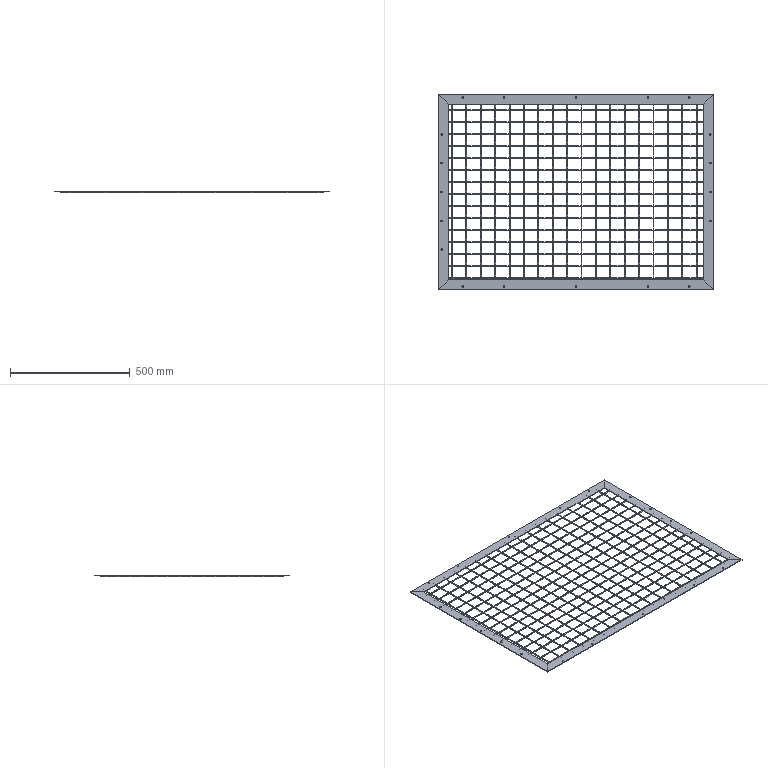Part | SolidWorks | features ICE 5, Extrusion 1, HoleWzd 1, WeldmentFeature 1 | 5 solids | 1274 faces | box 1144 x 813 x 7 mm | volume 815811 mm3 | cylinder 1184 | plane 90 | commonest cylinder face diameters 4 x1146 6.6 x38